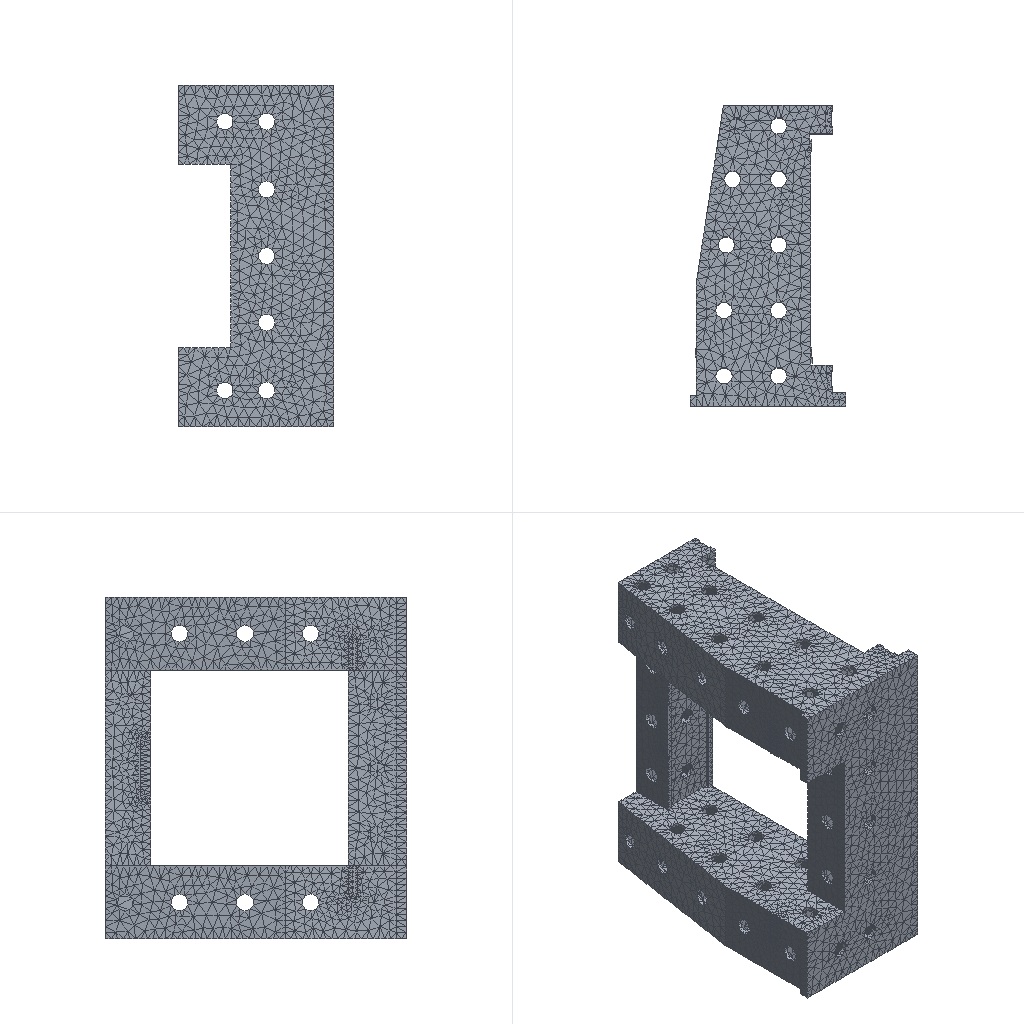Simulation study | ansys workbench
Set-up summary:
category,name,step,type,value,unit,region
solver,ansys_workbench
units,mm-N-s-tonne (MPa),,stated,"/units,MPA"
analysis,LS1,,modal,method=lanb; n_modes=15
load_step,LS1,LS1,modal
mesh,nodes,,,84641
mesh,elements,,,42630
element_type,SOLID187,,,42630
material,Structural Steel,,E,200000,tonne s^-2 mm^-1
material,Structural Steel,,nu,0.3
material,Structural Steel,,density,7.85e-09,tonne mm^-3
material,Structural Steel,,conductivity,60.5,tonne mm s^-3 C^-1
material,Structural Steel,,specific_heat,4.34e+08,mm^2 s^-2 C^-1
material,Structural Steel,,cte,1.2e-05,C^-1
material,Structural Steel,,permeability,10000
material,Structural Steel,,resistivity,0.00017,ohm mm
bc,Constant Zero Displacement X,model,fixed,[dofs=UX],,_DISPZEROUX
bc,Constant Zero Displacement Y,model,fixed,[dofs=UY],,_DISPZEROUY
bc,Constant Zero Displacement Z,model,fixed,[dofs=UZ],,_DISPZEROUZ
named_set,_DISPZEROUX,,node,2224
named_set,_DISPZEROUY,,node,2224
named_set,_DISPZEROUZ,,node,2224
Ansys APDL input file, long lists of numbers shortened:
/batch
/config,noeldb,1     ! force off writing results to database
*get,_wallstrt,active,,time,wall
! ANSYS input file written by Workbench version 2021 R1
! File used for geometry attach:
/title,wbnew--__ (E5)
! ****** Begin Custom Load Command Snippet ******
/COM, ACT Extensions:
/COM,     LSDYNA, 2021.1
/COM,
! ****** End   Custom Load Command Snippet ******
*DIM,_wb_ProjectScratch_dir,string,248
_wb_ProjectScratch_dir(1) = ''
*DIM,_wb_SolverFiles_dir,string,248
_wb_SolverFiles_dir(1) = ''
*DIM,_wb_userfiles_dir,string,248
_wb_userfiles_dir(1) = ''
/com,--- Data in consistent NMM units. See Solving Units in the help system for more information.
/units,MPA
/nopr
/wb,file,start              !  signify a WB generated input file
/prep7
! Turn off shape checking because checks already performed inside WB mesher.
! See help system for more information.
SHPP,OFF,,NOWARN
/nolist
etcon,set             ! allow ANSYS to choose best KEYOP's for 180x elements, resets any applicable keyopt to MAPDL defaults
/com,*********** Nodes for the whole assembly ***********
nblock,3,,93105
(1i9,3e20.9e3)
        1     8.051362184E+01     1.330000000E+03    -3.700000000E+02
! (84640 more lines like these left out)
-1
/wb,elem,start            !  set before creation of elements
/com,*********** Elements for Body 1 "lz-FreeParts|____-____18" ***********
et,1,187
eblock,19,solid,,42630
(19i9)
        1        1        1        1        0        0        0        0       10        0        1     1648     5602    13929    13862    23928    51855    23935    23933
! (85259 more lines like these left out)
-1
/wb,elem,end               !  done creating elements
/com,*********** Send User Defined Coordinate System(s) ***********
csys,0
toffst,273.15,  ! Temperature offset from absolute zero
/com,*********** Set Reference Temperature ***********
tref,22.
/wb,mat,start              !  starting to send materials
/com,*********** Send Materials ***********
Temperature = 'TEMP' ! Temperature
MP,DENS,1,7.85e-09,	! tonne mm^-3
MP,ALPX,1,1.2e-05,	! C^-1
MP,C,1,434000000,	! mm^2 s^-2 C^-1
MP,KXX,1,60.5,	! tonne mm s^-3 C^-1
MP,RSVX,1,0.00017,	! ohm mm
MP,EX,1,200000,	! tonne s^-2 mm^-1
MP,NUXY,1,0.3,
MP,MURX,1,10000,
/wb,mat,end                !  done sending materials
!************************* Model Summary ********************
!lz-FreeParts|____-____18,	结构钢,	matid,	1
!************************* End Model Summary ********************
! get the diagonal of the bounding box. Needed later for other things
*get,_xmin,node,,mnloc,x
*get,_ymin,node,,mnloc,y
*get,_zmin,node,,mnloc,z
*get,_xmax,node,,mxloc,x
*get,_ymax,node,,mxloc,y
*get,_zmax,node,,mxloc,z
_ASMDIAG=(_xmax-_xmin)*(_xmax-_xmin)+(_ymax-_ymin)*(_ymax-_ymin)+(_zmax-_zmin)*(_zmax-_zmin)
_ASMDIAG=SQRT(_ASMDIAG)
/wb,contact,start          !  starting to send contact
/wb,contact,end            !  done creating contacts
/golist
/wb,load,start             !  starting to send loads
/com,******* Constant Zero Displacement X *******
CMBLOCK,_DISPZEROUX,NODE,     2224
(8i10)
      1045      1046      1047      1048      1049      1050      1057      1058
! (277 more lines like these left out)
cmsel,s,_DISPZEROUX
d,all,ux,0
nsel,all
/com,******* Constant Zero Displacement Y *******
CMBLOCK,_DISPZEROUY,NODE,     2224
(8i10)
      1045      1046      1047      1048      1049      1050      1057      1058
! (277 more lines like these left out)
cmsel,s,_DISPZEROUY
d,all,uy,0
nsel,all
/com,******* Constant Zero Displacement Z *******
CMBLOCK,_DISPZEROUZ,NODE,     2224
(8i10)
      1045      1046      1047      1048      1049      1050      1057      1058
! (277 more lines like these left out)
cmsel,s,_DISPZEROUZ
d,all,uz,0
nsel,all
/gst,on,on
fini
*get,_numnode,node,0,count
*get,_numelem,elem,0,count
*get, _MAXELEMNUM, elem, 0, NUM, MAX
*get, _MAXNODENUM, node, 0, NUM, MAX
*get, _MAXELEMTYPE, etyp, 0, NUM, MAX
*get, _MAXREALCONST, real, 0, NUM, MAX
/go
/wb,load,end               !  done creating loads
/com,--- Number of total nodes = %_numnode%
/com,--- Number of contact elements = 0
/com,--- Number of spring elements = 0
/com,--- Number of bearing elements = 0
/com,--- Number of solid elements = 42630
/com,--- Number of condensed parts = 0
/com,--- Number of total elements = %_numelem%
*get,_wallbsol,active,,time,wall
/solu
antype,2                   ! modal analysis
_thickRatio=  0     ! Ratio of thick parts in the model
modopt,lanb,15
outres,erase
outres,all,none
outres,nsol,all
outres,etmp,all
mxpand                    ! default expand in case of complex solution
dmpopt,esav,no
dmpopt,emat,no
dmpopt,full,no
! *********** WB SOLVE COMMAND ***********
! check interactive state
*get,ANSINTER_,active,,int
*if,ANSINTER_,ne,0,then
/eof
*endif
solve
/com *************** Write FE CONNECTORS *********
CEWRITE,file,ce,,INTE
*get,_nmodalsolproc,active,0,numcpu
fini
/nopr
*get,_numnode,node,0,count
*get,_numelem,elem,0,count
*get, _MAXELEMNUM, elem, 0, NUM, MAX
*get, _MAXNODENUM, node, 0, NUM, MAX,,,INTERNAL
*get, _MAXELEMTYPE, etyp, 0, NUM, MAX
*get, _MAXREALCONST, real, 0, NUM, MAX
/gopr
*get,_wallasol,active,,time,wall
/post1
/nopr
*dim,_direction,CHAR,6,1
_direction(1) = 'X'
_direction(2) = 'Y'
_direction(3) = 'Z'
_direction(4) = 'ROTX'
_direction(5) = 'ROTY'
_direction(6) = 'ROTZ'
*get,_lastLS,active,0,set,LSTP
*get,_beginset,active,0,set,nset,first,_lastLS
*get,_endset,active,0,set,nset,last,_lastLS
_nummodes = 0
*if,_endset,gt,0,then
_nummodes = _endset - _beginset + 1
*endif
*do,i_mode,1,_nummodes
   *do,j_component,1,6
			*get,PFACT_%i_mode%_%j_component%,MODE,%i_mode%,PFACT,,DIREC,_direction(%j_component%)
   *enddo
*enddo
*dim,_tmdirection,CHAR,6,1
_tmdirection(1) = 'X'
_tmdirection(2) = 'Y'
_tmdirection(3) = 'Z'
_tmdirection(4) = 'X'
_tmdirection(5) = 'Y'
_tmdirection(6) = 'Z'
*do,j_component,1,6
    *if,j_component,gt,3,then
        *get,TOTALMASS_%j_component%,ELEM,0,IOR,_tmdirection(%j_component%)
    *else
        *get,TOTALMASS_%j_component%,ELEM,0,MTOT,_tmdirection(%j_component%)
    *endif
*enddo
/gopr
xmlo,ENCODING,ISO-8859-1
xmlo,parm
/xml,parm,xml
fini
/gopr
*get,_walldone,active,,time,wall
_preptime=(_wallbsol-_wallstrt)*3600
_solvtime=(_wallasol-_wallbsol)*3600
_posttime=(_walldone-_wallasol)*3600
_totaltim=(_walldone-_wallstrt)*3600
*get,_dlbratio,active,0,solu,dlbr
*get,_combtime,active,0,solu,comb
/com,--- Total number of nodes = %_numnode%
/com,--- Total number of elements = %_numelem%
/com,--- Element load balance ratio = %_dlbratio%
/com,--- Time to combine distributed files = %_combtime%
/wb,file,end               ! done with WB generated input
Results summary:
result,analyses[0].index,,,1
result,analyses[0].system,,,SYS-4
result,analyses[0].deck,,,deck.dat
result,analyses[0].solve_status,,,completed
result,analyses[0].analysis_type,,,modal
result,analyses[0].physics,,,mechanical
result,analyses[0].unit_system,,,"NMM: mm, ton, N, s, mV, mA, degC"
result,analyses[0].n_sets,,,15
result,analyses[0].modal_frequencies_hz[1],,,86.849
result,analyses[0].modal_frequencies_hz[2],,,91.341
result,analyses[0].modal_frequencies_hz[3],,,124.159
result,analyses[0].modal_frequencies_hz[4],,,253.584
result,analyses[0].modal_frequencies_hz[5],,,270.881
result,analyses[0].modal_frequencies_hz[6],,,352.212
result,analyses[0].modal_frequencies_hz[7],,,355.501
result,analyses[0].modal_frequencies_hz[8],,,359.595
result,analyses[0].modal_frequencies_hz[9],,,362.155
result,analyses[0].modal_frequencies_hz[10],,,417.395
result,analyses[0].modal_frequencies_hz[11],,,432.632
result,analyses[0].modal_frequencies_hz[12],,,467.719
result,analyses[0].modal_frequencies_hz[13],,,521.733
result,analyses[0].modal_frequencies_hz[14],,,562.732
result,analyses[0].modal_frequencies_hz[15],,,574.223
result,geometry_export[0][0],,,.step
result,geometry_export[0][1],,,ok
result,geometry_export[0][2],,,1